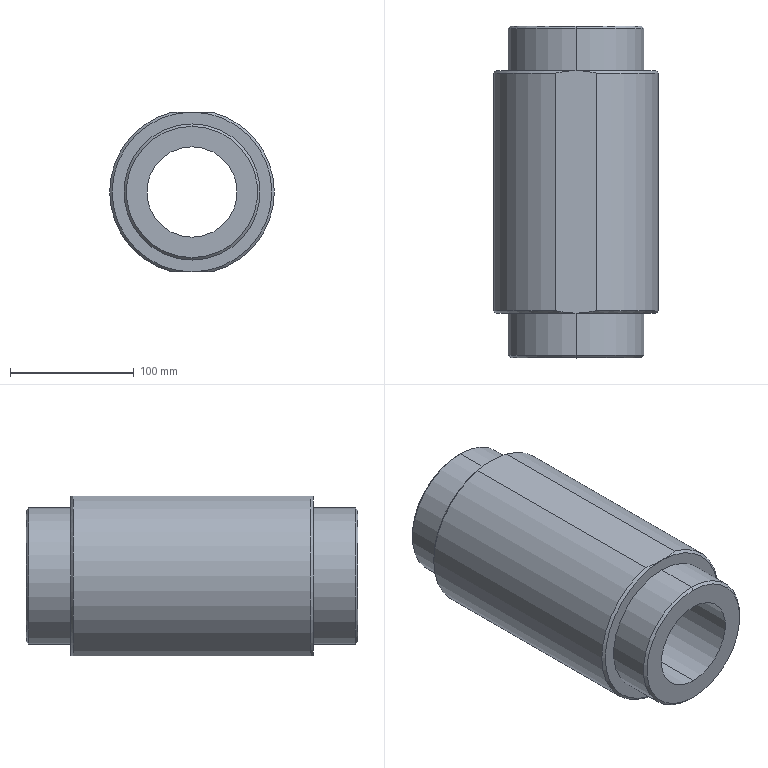Part | SolidWorks | features ICE 1, Revolution 1 | 1 solid | 22 faces | box 133 x 268 x 129 mm | volume 2265782 mm3 | cone 8 | cylinder 8 | plane 6 | commonest cylinder face diameters 110 x4 73 x2 133 x2
STEP:
#1=CARTESIAN_POINT('',(0.,0.,-53.));
#2=VERTEX_POINT('',#1);
#3=CARTESIAN_POINT('',(0.,0.,53.));
#4=VERTEX_POINT('',#3);
#5=CARTESIAN_POINT('',(0.,0.,0.));
#6=DIRECTION('',(0.,-1.,0.));
#7=DIRECTION('',(0.,0.,-1.));
#8=AXIS2_PLACEMENT_3D('',#5,#6,#7);
#9=CIRCLE('',#8,53.);
#10=EDGE_CURVE('',#2,#4,#9,.T.);
#11=ORIENTED_EDGE('',*,*,#10,.F.);
#12=CARTESIAN_POINT('',(0.,2.,-55.));
#13=VERTEX_POINT('',#12);
#14=CARTESIAN_POINT('',(0.,2.,-55.));
#15=DIRECTION('',(0.,0.7071,-0.7071));
#16=VECTOR('',#15,1000.);
#17=LINE('',#14,#16);
#18=EDGE_CURVE('',#2,#13,#17,.T.);
#19=ORIENTED_EDGE('',*,*,#18,.T.);
#20=CARTESIAN_POINT('',(0.,2.,55.));
#21=VERTEX_POINT('',#20);
#22=CARTESIAN_POINT('',(0.,2.,0.));
#23=DIRECTION('',(0.,-1.,0.));
#24=DIRECTION('',(0.,0.,-1.));
#25=AXIS2_PLACEMENT_3D('',#22,#23,#24);
#26=CIRCLE('',#25,55.);
#27=EDGE_CURVE('',#13,#21,#26,.T.);
#28=ORIENTED_EDGE('',*,*,#27,.T.);
#29=CARTESIAN_POINT('',(0.,2.,55.));
#30=DIRECTION('',(0.,0.7071,0.7071));
#31=VECTOR('',#30,1000.);
#32=LINE('',#29,#31);
#33=EDGE_CURVE('',#4,#21,#32,.T.);
#34=ORIENTED_EDGE('',*,*,#33,.F.);
#35=EDGE_LOOP('',(#11,#19,#28,#34));
#36=FACE_OUTER_BOUND('',#35,.T.);
#37=CARTESIAN_POINT('',(0.,2.,0.));
#38=DIRECTION('',(0.,1.,0.));
#39=DIRECTION('',(0.,0.,1.));
#40=AXIS2_PLACEMENT_3D('',#37,#38,#39);
#41=CONICAL_SURFACE('',#40,55.,0.7854);
#42=ADVANCED_FACE('',(#36),#41,.T.);
#43=CARTESIAN_POINT('',(0.,268.,36.5));
#44=VERTEX_POINT('',#43);
#45=CARTESIAN_POINT('',(0.,268.,-36.5));
#46=VERTEX_POINT('',#45);
#47=CARTESIAN_POINT('',(0.,268.,0.));
#48=DIRECTION('',(0.,-1.,0.));
#49=DIRECTION('',(0.,0.,-1.));
#50=AXIS2_PLACEMENT_3D('',#47,#48,#49);
#51=CIRCLE('',#50,36.5);
#52=EDGE_CURVE('',#44,#46,#51,.T.);
#53=ORIENTED_EDGE('',*,*,#52,.F.);
#54=CARTESIAN_POINT('',(0.,0.,36.5));
#55=VERTEX_POINT('',#54);
#56=CARTESIAN_POINT('',(0.,-26.656,36.5));
#57=DIRECTION('',(0.,-1.,0.));
#58=VECTOR('',#57,1000.);
#59=LINE('',#56,#58);
#60=EDGE_CURVE('',#44,#55,#59,.T.);
#61=ORIENTED_EDGE('',*,*,#60,.T.);
#62=CARTESIAN_POINT('',(0.,0.,-36.5));
#63=VERTEX_POINT('',#62);
#64=CARTESIAN_POINT('',(0.,0.,0.));
#65=DIRECTION('',(0.,-1.,0.));
#66=DIRECTION('',(0.,0.,-1.));
#67=AXIS2_PLACEMENT_3D('',#64,#65,#66);
#68=CIRCLE('',#67,36.5);
#69=EDGE_CURVE('',#55,#63,#68,.T.);
#70=ORIENTED_EDGE('',*,*,#69,.T.);
#71=CARTESIAN_POINT('',(0.,-26.656,-36.5));
#72=DIRECTION('',(0.,-1.,0.));
#73=VECTOR('',#72,1000.);
#74=LINE('',#71,#73);
#75=EDGE_CURVE('',#46,#63,#74,.T.);
#76=ORIENTED_EDGE('',*,*,#75,.F.);
#77=EDGE_LOOP('',(#53,#61,#70,#76));
#78=FACE_OUTER_BOUND('',#77,.T.);
#79=CARTESIAN_POINT('',(0.,-26.656,0.));
#80=DIRECTION('',(0.,-1.,0.));
#81=DIRECTION('',(0.,0.,-1.));
#82=AXIS2_PLACEMENT_3D('',#79,#80,#81);
#83=CYLINDRICAL_SURFACE('',#82,36.5);
#84=ADVANCED_FACE('',(#78),#83,.F.);
#85=CARTESIAN_POINT('',(0.,268.,-53.));
#86=VERTEX_POINT('',#85);
#87=CARTESIAN_POINT('',(0.,268.,53.));
#88=VERTEX_POINT('',#87);
#89=CARTESIAN_POINT('',(0.,268.,0.));
#90=DIRECTION('',(0.,-1.,0.));
#91=DIRECTION('',(0.,0.,-1.));
#92=AXIS2_PLACEMENT_3D('',#89,#90,#91);
#93=CIRCLE('',#92,53.);
#94=EDGE_CURVE('',#86,#88,#93,.T.);
#95=ORIENTED_EDGE('',*,*,#94,.T.);
#96=CARTESIAN_POINT('',(0.,266.,55.));
#97=VERTEX_POINT('',#96);
#98=CARTESIAN_POINT('',(0.,268.,53.));
#99=DIRECTION('',(0.,-0.7071,0.7071));
#100=VECTOR('',#99,1000.);
#101=LINE('',#98,#100);
#102=EDGE_CURVE('',#88,#97,#101,.T.);
#103=ORIENTED_EDGE('',*,*,#102,.T.);
#104=CARTESIAN_POINT('',(0.,266.,-55.));
#105=VERTEX_POINT('',#104);
#106=CARTESIAN_POINT('',(0.,266.,0.));
#107=DIRECTION('',(0.,-1.,0.));
#108=DIRECTION('',(0.,0.,-1.));
#109=AXIS2_PLACEMENT_3D('',#106,#107,#108);
#110=CIRCLE('',#109,55.);
#111=EDGE_CURVE('',#105,#97,#110,.T.);
#112=ORIENTED_EDGE('',*,*,#111,.F.);
#113=CARTESIAN_POINT('',(0.,268.,-53.));
#114=DIRECTION('',(0.,-0.7071,-0.7071));
#115=VECTOR('',#114,1000.);
#116=LINE('',#113,#115);
#117=EDGE_CURVE('',#86,#105,#116,.T.);
#118=ORIENTED_EDGE('',*,*,#117,.F.);
#119=EDGE_LOOP('',(#95,#103,#112,#118));
#120=FACE_OUTER_BOUND('',#119,.T.);
#121=CARTESIAN_POINT('',(0.,268.,0.));
#122=DIRECTION('',(0.,-1.,0.));
#123=DIRECTION('',(0.,0.,-1.));
#124=AXIS2_PLACEMENT_3D('',#121,#122,#123);
#125=CONICAL_SURFACE('',#124,53.,0.7854);
#126=ADVANCED_FACE('',(#120),#125,.T.);
#127=ORIENTED_EDGE('',*,*,#111,.T.);
#128=CARTESIAN_POINT('',(0.,232.,55.));
#129=VERTEX_POINT('',#128);
#130=CARTESIAN_POINT('',(0.,-26.656,55.));
#131=DIRECTION('',(0.,-1.,0.));
#132=VECTOR('',#131,1000.);
#133=LINE('',#130,#132);
#134=EDGE_CURVE('',#97,#129,#133,.T.);
#135=ORIENTED_EDGE('',*,*,#134,.T.);
#136=CARTESIAN_POINT('',(0.,232.,-55.));
#137=VERTEX_POINT('',#136);
#138=CARTESIAN_POINT('',(0.,232.,0.));
#139=DIRECTION('',(0.,-1.,0.));
#140=DIRECTION('',(0.,0.,-1.));
#141=AXIS2_PLACEMENT_3D('',#138,#139,#140);
#142=CIRCLE('',#141,55.);
#143=EDGE_CURVE('',#137,#129,#142,.T.);
#144=ORIENTED_EDGE('',*,*,#143,.F.);
#145=CARTESIAN_POINT('',(0.,-26.656,-55.));
#146=DIRECTION('',(0.,-1.,0.));
#147=VECTOR('',#146,1000.);
#148=LINE('',#145,#147);
#149=EDGE_CURVE('',#105,#137,#148,.T.);
#150=ORIENTED_EDGE('',*,*,#149,.F.);
#151=EDGE_LOOP('',(#127,#135,#144,#150));
#152=FACE_OUTER_BOUND('',#151,.T.);
#153=CARTESIAN_POINT('',(0.,-26.656,0.));
#154=DIRECTION('',(0.,-1.,0.));
#155=DIRECTION('',(0.,0.,-1.));
#156=AXIS2_PLACEMENT_3D('',#153,#154,#155);
#157=CYLINDRICAL_SURFACE('',#156,55.);
#158=ADVANCED_FACE('',(#152),#157,.T.);
#159=CARTESIAN_POINT('',(0.,36.,-55.));
#160=VERTEX_POINT('',#159);
#161=CARTESIAN_POINT('',(0.,36.,55.));
#162=VERTEX_POINT('',#161);
#163=CARTESIAN_POINT('',(0.,36.,0.));
#164=DIRECTION('',(0.,-1.,0.));
#165=DIRECTION('',(0.,0.,-1.));
#166=AXIS2_PLACEMENT_3D('',#163,#164,#165);
#167=CIRCLE('',#166,55.);
#168=EDGE_CURVE('',#160,#162,#167,.T.);
#169=ORIENTED_EDGE('',*,*,#168,.T.);
#170=CARTESIAN_POINT('',(0.,-26.656,55.));
#171=DIRECTION('',(0.,-1.,0.));
#172=VECTOR('',#171,1000.);
#173=LINE('',#170,#172);
#174=EDGE_CURVE('',#162,#21,#173,.T.);
#175=ORIENTED_EDGE('',*,*,#174,.T.);
#176=ORIENTED_EDGE('',*,*,#27,.F.);
#177=CARTESIAN_POINT('',(0.,-26.656,-55.));
#178=DIRECTION('',(0.,-1.,0.));
#179=VECTOR('',#178,1000.);
#180=LINE('',#177,#179);
#181=EDGE_CURVE('',#160,#13,#180,.T.);
#182=ORIENTED_EDGE('',*,*,#181,.F.);
#183=EDGE_LOOP('',(#169,#175,#176,#182));
#184=FACE_OUTER_BOUND('',#183,.T.);
#185=CARTESIAN_POINT('',(0.,-26.656,0.));
#186=DIRECTION('',(0.,-1.,0.));
#187=DIRECTION('',(0.,0.,-1.));
#188=AXIS2_PLACEMENT_3D('',#185,#186,#187);
#189=CYLINDRICAL_SURFACE('',#188,55.);
#190=ADVANCED_FACE('',(#184),#189,.T.);
#191=CARTESIAN_POINT('',(-16.186,38.,64.5));
#192=VERTEX_POINT('',#191);
#193=CARTESIAN_POINT('',(-16.186,38.,-64.5));
#194=VERTEX_POINT('',#193);
#195=CARTESIAN_POINT('',(0.,38.,0.));
#196=DIRECTION('',(0.,-1.,0.));
#197=DIRECTION('',(0.,0.,-1.));
#198=AXIS2_PLACEMENT_3D('',#195,#196,#197);
#199=CIRCLE('',#198,66.5);
#200=EDGE_CURVE('',#192,#194,#199,.T.);
#201=ORIENTED_EDGE('',*,*,#200,.T.);
#202=CARTESIAN_POINT('',(0.,36.,-64.5));
#203=VERTEX_POINT('',#202);
#204=CARTESIAN_POINT('',(-16.186,38.,-64.5));
#205=CARTESIAN_POINT('',(-14.864,37.678,-64.5));
#206=CARTESIAN_POINT('',(-13.529,37.39,-64.5));
#207=CARTESIAN_POINT('',(-10.832,36.89,-64.5));
#208=CARTESIAN_POINT('',(-9.482,36.679,-64.5));
#209=CARTESIAN_POINT('',(-5.426,36.172,-64.5));
#210=CARTESIAN_POINT('',(-2.716,36.,-64.5));
#211=CARTESIAN_POINT('',(0.,36.,-64.5));
#212=B_SPLINE_CURVE_WITH_KNOTS('',3,(#204,#205,#206,#207,#208,#209,#210,#211),.UNSPECIFIED.,.F.,.F.,(4,2,2,4),(0.02514,0.0292,0.03326,0.04137),.UNSPECIFIED.);
#213=EDGE_CURVE('',#194,#203,#212,.T.);
#214=ORIENTED_EDGE('',*,*,#213,.T.);
#215=CARTESIAN_POINT('',(0.,36.,64.5));
#216=VERTEX_POINT('',#215);
#217=CARTESIAN_POINT('',(0.,36.,0.));
#218=DIRECTION('',(0.,-1.,0.));
#219=DIRECTION('',(0.,0.,-1.));
#220=AXIS2_PLACEMENT_3D('',#217,#218,#219);
#221=CIRCLE('',#220,64.5);
#222=EDGE_CURVE('',#216,#203,#221,.T.);
#223=ORIENTED_EDGE('',*,*,#222,.F.);
#224=CARTESIAN_POINT('',(0.,36.,64.5));
#225=CARTESIAN_POINT('',(-2.716,36.,64.5));
#226=CARTESIAN_POINT('',(-5.426,36.172,64.5));
#227=CARTESIAN_POINT('',(-9.482,36.679,64.5));
#228=CARTESIAN_POINT('',(-10.832,36.89,64.5));
#229=CARTESIAN_POINT('',(-13.529,37.39,64.5));
#230=CARTESIAN_POINT('',(-14.864,37.678,64.5));
#231=CARTESIAN_POINT('',(-16.186,38.,64.5));
#232=B_SPLINE_CURVE_WITH_KNOTS('',3,(#224,#225,#226,#227,#228,#229,#230,#231),.UNSPECIFIED.,.F.,.F.,(4,2,2,4),(0.03445,0.04256,0.04661,0.05066),.UNSPECIFIED.);
#233=EDGE_CURVE('',#216,#192,#232,.T.);
#234=ORIENTED_EDGE('',*,*,#233,.T.);
#235=EDGE_LOOP('',(#201,#214,#223,#234));
#236=FACE_OUTER_BOUND('',#235,.T.);
#237=CARTESIAN_POINT('',(0.,38.,0.));
#238=DIRECTION('',(0.,1.,0.));
#239=DIRECTION('',(0.,0.,1.));
#240=AXIS2_PLACEMENT_3D('',#237,#238,#239);
#241=CONICAL_SURFACE('',#240,66.5,0.7854);
#242=ADVANCED_FACE('',(#236),#241,.T.);
#243=CARTESIAN_POINT('',(-16.186,230.,64.5));
#244=VERTEX_POINT('',#243);
#245=CARTESIAN_POINT('',(-16.186,230.,-64.5));
#246=VERTEX_POINT('',#245);
#247=CARTESIAN_POINT('',(0.,230.,0.));
#248=DIRECTION('',(0.,-1.,0.));
#249=DIRECTION('',(0.,0.,-1.));
#250=AXIS2_PLACEMENT_3D('',#247,#248,#249);
#251=CIRCLE('',#250,66.5);
#252=EDGE_CURVE('',#244,#246,#251,.T.);
#253=ORIENTED_EDGE('',*,*,#252,.T.);
#254=CARTESIAN_POINT('',(-16.186,268.,-64.5));
#255=DIRECTION('',(0.,-1.,0.));
#256=VECTOR('',#255,1000.);
#257=LINE('',#254,#256);
#258=EDGE_CURVE('',#246,#194,#257,.T.);
#259=ORIENTED_EDGE('',*,*,#258,.T.);
#260=ORIENTED_EDGE('',*,*,#200,.F.);
#261=CARTESIAN_POINT('',(-16.186,268.,64.5));
#262=DIRECTION('',(0.,-1.,0.));
#263=VECTOR('',#262,1000.);
#264=LINE('',#261,#263);
#265=EDGE_CURVE('',#244,#192,#264,.T.);
#266=ORIENTED_EDGE('',*,*,#265,.F.);
#267=EDGE_LOOP('',(#253,#259,#260,#266));
#268=FACE_OUTER_BOUND('',#267,.T.);
#269=CARTESIAN_POINT('',(0.,-26.656,0.));
#270=DIRECTION('',(0.,-1.,0.));
#271=DIRECTION('',(0.,0.,-1.));
#272=AXIS2_PLACEMENT_3D('',#269,#270,#271);
#273=CYLINDRICAL_SURFACE('',#272,66.5);
#274=ADVANCED_FACE('',(#268),#273,.T.);
#275=CARTESIAN_POINT('',(16.186,230.,-64.5));
#276=VERTEX_POINT('',#275);
#277=CARTESIAN_POINT('',(16.186,230.,64.5));
#278=VERTEX_POINT('',#277);
#279=CARTESIAN_POINT('',(0.,230.,0.));
#280=DIRECTION('',(0.,-1.,0.));
#281=DIRECTION('',(0.,0.,-1.));
#282=AXIS2_PLACEMENT_3D('',#279,#280,#281);
#283=CIRCLE('',#282,66.5);
#284=EDGE_CURVE('',#276,#278,#283,.T.);
#285=ORIENTED_EDGE('',*,*,#284,.F.);
#286=CARTESIAN_POINT('',(0.,232.,-64.5));
#287=VERTEX_POINT('',#286);
#288=CARTESIAN_POINT('',(16.186,230.,-64.5));
#289=CARTESIAN_POINT('',(13.557,230.64,-64.5));
#290=CARTESIAN_POINT('',(10.886,231.143,-64.5));
#291=CARTESIAN_POINT('',(7.489,231.57,-64.5));
#292=CARTESIAN_POINT('',(6.806,231.645,-64.5));
#293=CARTESIAN_POINT('',(5.442,231.774,-64.5));
#294=CARTESIAN_POINT('',(4.761,231.828,-64.5));
#295=CARTESIAN_POINT('',(2.719,231.957,-64.5));
#296=CARTESIAN_POINT('',(1.359,232.,-64.5));
#297=CARTESIAN_POINT('',(0.,232.,-64.5));
#298=B_SPLINE_CURVE_WITH_KNOTS('',3,(#288,#289,#290,#291,#292,#293,#294,#295,#296,#297),.UNSPECIFIED.,.F.,.F.,(4,2,2,2,4),(0.01823,0.02634,0.02837,0.03039,0.03445),.UNSPECIFIED.);
#299=EDGE_CURVE('',#276,#287,#298,.T.);
#300=ORIENTED_EDGE('',*,*,#299,.T.);
#301=CARTESIAN_POINT('',(0.,232.,64.5));
#302=VERTEX_POINT('',#301);
#303=CARTESIAN_POINT('',(0.,232.,0.));
#304=DIRECTION('',(0.,-1.,0.));
#305=DIRECTION('',(0.,0.,-1.));
#306=AXIS2_PLACEMENT_3D('',#303,#304,#305);
#307=CIRCLE('',#306,64.5);
#308=EDGE_CURVE('',#287,#302,#307,.T.);
#309=ORIENTED_EDGE('',*,*,#308,.T.);
#310=CARTESIAN_POINT('',(0.,232.,64.5));
#311=CARTESIAN_POINT('',(1.359,232.,64.5));
#312=CARTESIAN_POINT('',(2.719,231.957,64.5));
#313=CARTESIAN_POINT('',(4.761,231.828,64.5));
#314=CARTESIAN_POINT('',(5.442,231.774,64.5));
#315=CARTESIAN_POINT('',(6.806,231.645,64.5));
#316=CARTESIAN_POINT('',(7.489,231.57,64.5));
#317=CARTESIAN_POINT('',(10.886,231.143,64.5));
#318=CARTESIAN_POINT('',(13.557,230.64,64.5));
#319=CARTESIAN_POINT('',(16.186,230.,64.5));
#320=B_SPLINE_CURVE_WITH_KNOTS('',3,(#310,#311,#312,#313,#314,#315,#316,#317,#318,#319),.UNSPECIFIED.,.F.,.F.,(4,2,2,2,4),(0.04137,0.04543,0.04746,0.04949,0.0576),.UNSPECIFIED.);
#321=EDGE_CURVE('',#302,#278,#320,.T.);
#322=ORIENTED_EDGE('',*,*,#321,.T.);
#323=EDGE_LOOP('',(#285,#300,#309,#322));
#324=FACE_OUTER_BOUND('',#323,.T.);
#325=CARTESIAN_POINT('',(0.,232.,0.));
#326=DIRECTION('',(0.,-1.,0.));
#327=DIRECTION('',(0.,0.,-1.));
#328=AXIS2_PLACEMENT_3D('',#325,#326,#327);
#329=CONICAL_SURFACE('',#328,64.5,0.7854);
#330=ADVANCED_FACE('',(#324),#329,.T.);
#331=ORIENTED_EDGE('',*,*,#174,.F.);
#332=CARTESIAN_POINT('',(0.,36.,0.));
#333=DIRECTION('',(0.,-1.,0.));
#334=DIRECTION('',(0.,0.,-1.));
#335=AXIS2_PLACEMENT_3D('',#332,#333,#334);
#336=CIRCLE('',#335,55.);
#337=EDGE_CURVE('',#162,#160,#336,.T.);
#338=ORIENTED_EDGE('',*,*,#337,.T.);
#339=ORIENTED_EDGE('',*,*,#181,.T.);
#340=CARTESIAN_POINT('',(0.,2.,0.));
#341=DIRECTION('',(0.,-1.,0.));
#342=DIRECTION('',(0.,0.,-1.));
#343=AXIS2_PLACEMENT_3D('',#340,#341,#342);
#344=CIRCLE('',#343,55.);
#345=EDGE_CURVE('',#21,#13,#344,.T.);
#346=ORIENTED_EDGE('',*,*,#345,.F.);
#347=EDGE_LOOP('',(#331,#338,#339,#346));
#348=FACE_OUTER_BOUND('',#347,.T.);
#349=CARTESIAN_POINT('',(0.,-26.656,0.));
#350=DIRECTION('',(0.,-1.,0.));
#351=DIRECTION('',(0.,0.,-1.));
#352=AXIS2_PLACEMENT_3D('',#349,#350,#351);
#353=CYLINDRICAL_SURFACE('',#352,55.);
#354=ADVANCED_FACE('',(#348),#353,.T.);
#355=ORIENTED_EDGE('',*,*,#168,.F.);
#356=ORIENTED_EDGE('',*,*,#337,.F.);
#357=EDGE_LOOP('',(#355,#356));
#358=FACE_BOUND('',#357,.T.);
#359=ORIENTED_EDGE('',*,*,#222,.T.);
#360=CARTESIAN_POINT('',(0.,36.,0.));
#361=DIRECTION('',(0.,-1.,0.));
#362=DIRECTION('',(0.,0.,-1.));
#363=AXIS2_PLACEMENT_3D('',#360,#361,#362);
#364=CIRCLE('',#363,64.5);
#365=EDGE_CURVE('',#203,#216,#364,.T.);
#366=ORIENTED_EDGE('',*,*,#365,.T.);
#367=EDGE_LOOP('',(#359,#366));
#368=FACE_OUTER_BOUND('',#367,.T.);
#369=CARTESIAN_POINT('',(-64.5,36.,0.));
#370=DIRECTION('',(0.,1.,0.));
#371=DIRECTION('',(0.,0.,1.));
#372=AXIS2_PLACEMENT_3D('',#369,#370,#371);
#373=PLANE('',#372);
#374=ADVANCED_FACE('',(#358,#368),#373,.F.);
#375=ORIENTED_EDGE('',*,*,#365,.F.);
#376=CARTESIAN_POINT('',(16.186,38.,-64.5));
#377=VERTEX_POINT('',#376);
#378=CARTESIAN_POINT('',(0.,36.,-64.5));
#379=CARTESIAN_POINT('',(1.359,36.,-64.5));
#380=CARTESIAN_POINT('',(2.719,36.043,-64.5));
#381=CARTESIAN_POINT('',(4.761,36.172,-64.5));
#382=CARTESIAN_POINT('',(5.442,36.226,-64.5));
#383=CARTESIAN_POINT('',(6.806,36.355,-64.5));
#384=CARTESIAN_POINT('',(7.489,36.43,-64.5));
#385=CARTESIAN_POINT('',(10.886,36.857,-64.5));
#386=CARTESIAN_POINT('',(13.557,37.36,-64.5));
#387=CARTESIAN_POINT('',(16.186,38.,-64.5));
#388=B_SPLINE_CURVE_WITH_KNOTS('',3,(#378,#379,#380,#381,#382,#383,#384,#385,#386,#387),.UNSPECIFIED.,.F.,.F.,(4,2,2,2,4),(0.04137,0.04543,0.04746,0.04949,0.0576),.UNSPECIFIED.);
#389=EDGE_CURVE('',#203,#377,#388,.T.);
#390=ORIENTED_EDGE('',*,*,#389,.T.);
#391=CARTESIAN_POINT('',(16.186,38.,64.5));
#392=VERTEX_POINT('',#391);
#393=CARTESIAN_POINT('',(0.,38.,0.));
#394=DIRECTION('',(0.,-1.,0.));
#395=DIRECTION('',(0.,0.,-1.));
#396=AXIS2_PLACEMENT_3D('',#393,#394,#395);
#397=CIRCLE('',#396,66.5);
#398=EDGE_CURVE('',#377,#392,#397,.T.);
#399=ORIENTED_EDGE('',*,*,#398,.T.);
#400=CARTESIAN_POINT('',(16.186,38.,64.5));
#401=CARTESIAN_POINT('',(13.557,37.36,64.5));
#402=CARTESIAN_POINT('',(10.886,36.857,64.5));
#403=CARTESIAN_POINT('',(7.489,36.43,64.5));
#404=CARTESIAN_POINT('',(6.806,36.355,64.5));
#405=CARTESIAN_POINT('',(5.442,36.226,64.5));
#406=CARTESIAN_POINT('',(4.761,36.172,64.5));
#407=CARTESIAN_POINT('',(2.719,36.043,64.5));
#408=CARTESIAN_POINT('',(1.359,36.,64.5));
#409=CARTESIAN_POINT('',(0.,36.,64.5));
#410=B_SPLINE_CURVE_WITH_KNOTS('',3,(#400,#401,#402,#403,#404,#405,#406,#407,#408,#409),.UNSPECIFIED.,.F.,.F.,(4,2,2,2,4),(0.01823,0.02634,0.02837,0.03039,0.03445),.UNSPECIFIED.);
#411=EDGE_CURVE('',#392,#216,#410,.T.);
#412=ORIENTED_EDGE('',*,*,#411,.T.);
#413=EDGE_LOOP('',(#375,#390,#399,#412));
#414=FACE_OUTER_BOUND('',#413,.T.);
#415=CARTESIAN_POINT('',(0.,38.,0.));
#416=DIRECTION('',(0.,1.,0.));
#417=DIRECTION('',(0.,0.,1.));
#418=AXIS2_PLACEMENT_3D('',#415,#416,#417);
#419=CONICAL_SURFACE('',#418,66.5,0.7854);
#420=ADVANCED_FACE('',(#414),#419,.T.);
#421=ORIENTED_EDGE('',*,*,#398,.F.);
#422=CARTESIAN_POINT('',(16.186,268.,-64.5));
#423=DIRECTION('',(0.,-1.,0.));
#424=VECTOR('',#423,1000.);
#425=LINE('',#422,#424);
#426=EDGE_CURVE('',#276,#377,#425,.T.);
#427=ORIENTED_EDGE('',*,*,#426,.F.);
#428=ORIENTED_EDGE('',*,*,#284,.T.);
#429=CARTESIAN_POINT('',(16.186,268.,64.5));
#430=DIRECTION('',(0.,-1.,0.));
#431=VECTOR('',#430,1000.);
#432=LINE('',#429,#431);
#433=EDGE_CURVE('',#278,#392,#432,.T.);
#434=ORIENTED_EDGE('',*,*,#433,.T.);
#435=EDGE_LOOP('',(#421,#427,#428,#434));
#436=FACE_OUTER_BOUND('',#435,.T.);
#437=CARTESIAN_POINT('',(0.,-26.656,0.));
#438=DIRECTION('',(0.,-1.,0.));
#439=DIRECTION('',(0.,0.,-1.));
#440=AXIS2_PLACEMENT_3D('',#437,#438,#439);
#441=CYLINDRICAL_SURFACE('',#440,66.5);
#442=ADVANCED_FACE('',(#436),#441,.T.);
#443=CARTESIAN_POINT('',(0.,232.,0.));
#444=DIRECTION('',(0.,-1.,0.));
#445=DIRECTION('',(0.,0.,-1.));
#446=AXIS2_PLACEMENT_3D('',#443,#444,#445);
#447=CIRCLE('',#446,64.5);
#448=EDGE_CURVE('',#302,#287,#447,.T.);
#449=ORIENTED_EDGE('',*,*,#448,.T.);
#450=CARTESIAN_POINT('',(0.,232.,-64.5));
#451=CARTESIAN_POINT('',(-2.716,232.,-64.5));
#452=CARTESIAN_POINT('',(-5.426,231.828,-64.5));
#453=CARTESIAN_POINT('',(-9.482,231.321,-64.5));
#454=CARTESIAN_POINT('',(-10.832,231.11,-64.5));
#455=CARTESIAN_POINT('',(-13.529,230.61,-64.5));
#456=CARTESIAN_POINT('',(-14.864,230.322,-64.5));
#457=CARTESIAN_POINT('',(-16.186,230.,-64.5));
#458=B_SPLINE_CURVE_WITH_KNOTS('',3,(#450,#451,#452,#453,#454,#455,#456,#457),.UNSPECIFIED.,.F.,.F.,(4,2,2,4),(0.03445,0.04256,0.04661,0.05066),.UNSPECIFIED.);
#459=EDGE_CURVE('',#287,#246,#458,.T.);
#460=ORIENTED_EDGE('',*,*,#459,.T.);
#461=ORIENTED_EDGE('',*,*,#252,.F.);
#462=CARTESIAN_POINT('',(-16.186,230.,64.5));
#463=CARTESIAN_POINT('',(-14.864,230.322,64.5));
#464=CARTESIAN_POINT('',(-13.529,230.61,64.5));
#465=CARTESIAN_POINT('',(-10.832,231.11,64.5));
#466=CARTESIAN_POINT('',(-9.482,231.321,64.5));
#467=CARTESIAN_POINT('',(-5.426,231.828,64.5));
#468=CARTESIAN_POINT('',(-2.716,232.,64.5));
#469=CARTESIAN_POINT('',(0.,232.,64.5));
#470=B_SPLINE_CURVE_WITH_KNOTS('',3,(#462,#463,#464,#465,#466,#467,#468,#469),.UNSPECIFIED.,.F.,.F.,(4,2,2,4),(0.02514,0.0292,0.03326,0.04137),.UNSPECIFIED.);
#471=EDGE_CURVE('',#244,#302,#470,.T.);
#472=ORIENTED_EDGE('',*,*,#471,.T.);
#473=EDGE_LOOP('',(#449,#460,#461,#472));
#474=FACE_OUTER_BOUND('',#473,.T.);
#475=CARTESIAN_POINT('',(0.,232.,0.));
#476=DIRECTION('',(0.,-1.,0.));
#477=DIRECTION('',(0.,0.,-1.));
#478=AXIS2_PLACEMENT_3D('',#475,#476,#477);
#479=CONICAL_SURFACE('',#478,64.5,0.7854);
#480=ADVANCED_FACE('',(#474),#479,.T.);
#481=ORIENTED_EDGE('',*,*,#448,.F.);
#482=ORIENTED_EDGE('',*,*,#308,.F.);
#483=EDGE_LOOP('',(#481,#482));
#484=FACE_OUTER_BOUND('',#483,.T.);
#485=ORIENTED_EDGE('',*,*,#143,.T.);
#486=CARTESIAN_POINT('',(0.,232.,0.));
#487=DIRECTION('',(0.,-1.,0.));
#488=DIRECTION('',(0.,0.,-1.));
#489=AXIS2_PLACEMENT_3D('',#486,#487,#488);
#490=CIRCLE('',#489,55.);
#491=EDGE_CURVE('',#129,#137,#490,.T.);
#492=ORIENTED_EDGE('',*,*,#491,.T.);
#493=EDGE_LOOP('',(#485,#492));
#494=FACE_BOUND('',#493,.T.);
#495=CARTESIAN_POINT('',(-64.5,232.,0.));
#496=DIRECTION('',(0.,-1.,0.));
#497=DIRECTION('',(0.,0.,-1.));
#498=AXIS2_PLACEMENT_3D('',#495,#496,#497);
#499=PLANE('',#498);
#500=ADVANCED_FACE('',(#484,#494),#499,.F.);
#501=ORIENTED_EDGE('',*,*,#134,.F.);
#502=CARTESIAN_POINT('',(0.,266.,0.));
#503=DIRECTION('',(0.,-1.,0.));
#504=DIRECTION('',(0.,0.,-1.));
#505=AXIS2_PLACEMENT_3D('',#502,#503,#504);
#506=CIRCLE('',#505,55.);
#507=EDGE_CURVE('',#97,#105,#506,.T.);
#508=ORIENTED_EDGE('',*,*,#507,.T.);
#509=ORIENTED_EDGE('',*,*,#149,.T.);
#510=ORIENTED_EDGE('',*,*,#491,.F.);
#511=EDGE_LOOP('',(#501,#508,#509,#510));
#512=FACE_OUTER_BOUND('',#511,.T.);
#513=CARTESIAN_POINT('',(0.,-26.656,0.));
#514=DIRECTION('',(0.,-1.,0.));
#515=DIRECTION('',(0.,0.,-1.));
#516=AXIS2_PLACEMENT_3D('',#513,#514,#515);
#517=CYLINDRICAL_SURFACE('',#516,55.);
#518=ADVANCED_FACE('',(#512),#517,.T.);
#519=ORIENTED_EDGE('',*,*,#102,.F.);
#520=CARTESIAN_POINT('',(0.,268.,0.));
#521=DIRECTION('',(0.,-1.,0.));
#522=DIRECTION('',(0.,0.,-1.));
#523=AXIS2_PLACEMENT_3D('',#520,#521,#522);
#524=CIRCLE('',#523,53.);
#525=EDGE_CURVE('',#88,#86,#524,.T.);
#526=ORIENTED_EDGE('',*,*,#525,.T.);
#527=ORIENTED_EDGE('',*,*,#117,.T.);
#528=ORIENTED_EDGE('',*,*,#507,.F.);
#529=EDGE_LOOP('',(#519,#526,#527,#528));
#530=FACE_OUTER_BOUND('',#529,.T.);
#531=CARTESIAN_POINT('',(0.,268.,0.));
#532=DIRECTION('',(0.,-1.,0.));
#533=DIRECTION('',(0.,0.,-1.));
#534=AXIS2_PLACEMENT_3D('',#531,#532,#533);
#535=CONICAL_SURFACE('',#534,53.,0.7854);
#536=ADVANCED_FACE('',(#530),#535,.T.);
#537=ORIENTED_EDGE('',*,*,#94,.F.);
#538=ORIENTED_EDGE('',*,*,#525,.F.);
#539=EDGE_LOOP('',(#537,#538));
#540=FACE_OUTER_BOUND('',#539,.T.);
#541=CARTESIAN_POINT('',(0.,268.,0.));
#542=DIRECTION('',(0.,-1.,0.));
#543=DIRECTION('',(0.,0.,-1.));
#544=AXIS2_PLACEMENT_3D('',#541,#542,#543);
#545=CIRCLE('',#544,36.5);
#546=EDGE_CURVE('',#46,#44,#545,.T.);
#547=ORIENTED_EDGE('',*,*,#546,.T.);
#548=ORIENTED_EDGE('',*,*,#52,.T.);
#549=EDGE_LOOP('',(#547,#548));
#550=FACE_BOUND('',#549,.T.);
#551=CARTESIAN_POINT('',(-53.,268.,0.));
#552=DIRECTION('',(0.,-1.,0.));
#553=DIRECTION('',(0.,0.,-1.));
#554=AXIS2_PLACEMENT_3D('',#551,#552,#553);
#555=PLANE('',#554);
#556=ADVANCED_FACE('',(#540,#550),#555,.F.);
#557=ORIENTED_EDGE('',*,*,#60,.F.);
#558=ORIENTED_EDGE('',*,*,#546,.F.);
#559=ORIENTED_EDGE('',*,*,#75,.T.);
#560=CARTESIAN_POINT('',(0.,0.,0.));
#561=DIRECTION('',(0.,-1.,0.));
#562=DIRECTION('',(0.,0.,-1.));
#563=AXIS2_PLACEMENT_3D('',#560,#561,#562);
#564=CIRCLE('',#563,36.5);
#565=EDGE_CURVE('',#63,#55,#564,.T.);
#566=ORIENTED_EDGE('',*,*,#565,.T.);
#567=EDGE_LOOP('',(#557,#558,#559,#566));
#568=FACE_OUTER_BOUND('',#567,.T.);
#569=CARTESIAN_POINT('',(0.,-26.656,0.));
#570=DIRECTION('',(0.,-1.,0.));
#571=DIRECTION('',(0.,0.,-1.));
#572=AXIS2_PLACEMENT_3D('',#569,#570,#571);
#573=CYLINDRICAL_SURFACE('',#572,36.5);
#574=ADVANCED_FACE('',(#568),#573,.F.);
#575=ORIENTED_EDGE('',*,*,#565,.F.);
#576=ORIENTED_EDGE('',*,*,#69,.F.);
#577=EDGE_LOOP('',(#575,#576));
#578=FACE_BOUND('',#577,.T.);
#579=CARTESIAN_POINT('',(0.,0.,0.));
#580=DIRECTION('',(0.,-1.,0.));
#581=DIRECTION('',(0.,0.,-1.));
#582=AXIS2_PLACEMENT_3D('',#579,#580,#581);
#583=CIRCLE('',#582,53.);
#584=EDGE_CURVE('',#4,#2,#583,.T.);
#585=ORIENTED_EDGE('',*,*,#584,.T.);
#586=ORIENTED_EDGE('',*,*,#10,.T.);
#587=EDGE_LOOP('',(#585,#586));
#588=FACE_OUTER_BOUND('',#587,.T.);
#589=CARTESIAN_POINT('',(-36.5,0.,0.));
#590=DIRECTION('',(0.,1.,0.));
#591=DIRECTION('',(0.,0.,1.));
#592=AXIS2_PLACEMENT_3D('',#589,#590,#591);
#593=PLANE('',#592);
#594=ADVANCED_FACE('',(#578,#588),#593,.F.);
#595=ORIENTED_EDGE('',*,*,#18,.F.);
#596=ORIENTED_EDGE('',*,*,#584,.F.);
#597=ORIENTED_EDGE('',*,*,#33,.T.);
#598=ORIENTED_EDGE('',*,*,#345,.T.);
#599=EDGE_LOOP('',(#595,#596,#597,#598));
#600=FACE_OUTER_BOUND('',#599,.T.);
#601=CARTESIAN_POINT('',(0.,2.,0.));
#602=DIRECTION('',(0.,1.,0.));
#603=DIRECTION('',(0.,0.,1.));
#604=AXIS2_PLACEMENT_3D('',#601,#602,#603);
#605=CONICAL_SURFACE('',#604,55.,0.7854);
#606=ADVANCED_FACE('',(#600),#605,.T.);
#607=ORIENTED_EDGE('',*,*,#433,.F.);
#608=ORIENTED_EDGE('',*,*,#321,.F.);
#609=ORIENTED_EDGE('',*,*,#471,.F.);
#610=ORIENTED_EDGE('',*,*,#265,.T.);
#611=ORIENTED_EDGE('',*,*,#233,.F.);
#612=ORIENTED_EDGE('',*,*,#411,.F.);
#613=EDGE_LOOP('',(#607,#608,#609,#610,#611,#612));
#614=FACE_OUTER_BOUND('',#613,.T.);
#615=CARTESIAN_POINT('',(-16.186,268.,64.5));
#616=DIRECTION('',(0.,0.,-1.));
#617=DIRECTION('',(-1.,0.,0.));
#618=AXIS2_PLACEMENT_3D('',#615,#616,#617);
#619=PLANE('',#618);
#620=ADVANCED_FACE('',(#614),#619,.F.);
#621=ORIENTED_EDGE('',*,*,#258,.F.);
#622=ORIENTED_EDGE('',*,*,#459,.F.);
#623=ORIENTED_EDGE('',*,*,#299,.F.);
#624=ORIENTED_EDGE('',*,*,#426,.T.);
#625=ORIENTED_EDGE('',*,*,#389,.F.);
#626=ORIENTED_EDGE('',*,*,#213,.F.);
#627=EDGE_LOOP('',(#621,#622,#623,#624,#625,#626));
#628=FACE_OUTER_BOUND('',#627,.T.);
#629=CARTESIAN_POINT('',(-16.186,268.,-64.5));
#630=DIRECTION('',(0.,0.,1.));
#631=DIRECTION('',(1.,0.,0.));
#632=AXIS2_PLACEMENT_3D('',#629,#630,#631);
#633=PLANE('',#632);
#634=ADVANCED_FACE('',(#628),#633,.F.);
#635=CLOSED_SHELL('',(#42,#84,#126,#158,#190,#242,#274,#330,#354,#374,#420,#442,#480,#500,#518,#536,#556,#574,#594,#606,#620,#634));
#636=MANIFOLD_SOLID_BREP('',#635);
#637=CARTESIAN_POINT('',(0.,0.,0.));
#638=DIRECTION('',(0.,0.,1.));
#639=DIRECTION('',(1.,0.,0.));
#640=AXIS2_PLACEMENT_3D('',#637,#638,#639);
#641=(LENGTH_UNIT()NAMED_UNIT(*)SI_UNIT(.MILLI.,.METRE.));
#642=UNCERTAINTY_MEASURE_WITH_UNIT(LENGTH_MEASURE(0.00001),#641,'','');
#643=(NAMED_UNIT(*)PLANE_ANGLE_UNIT()SI_UNIT($,.RADIAN.));
#644=(NAMED_UNIT(*)SI_UNIT($,.STERADIAN.)SOLID_ANGLE_UNIT());
#645=(GEOMETRIC_REPRESENTATION_CONTEXT(3)GLOBAL_UNCERTAINTY_ASSIGNED_CONTEXT((#642))GLOBAL_UNIT_ASSIGNED_CONTEXT((#641,#643,#644))REPRESENTATION_CONTEXT('',''));
#646=ADVANCED_BREP_SHAPE_REPRESENTATION('',(#636,#640),#645);